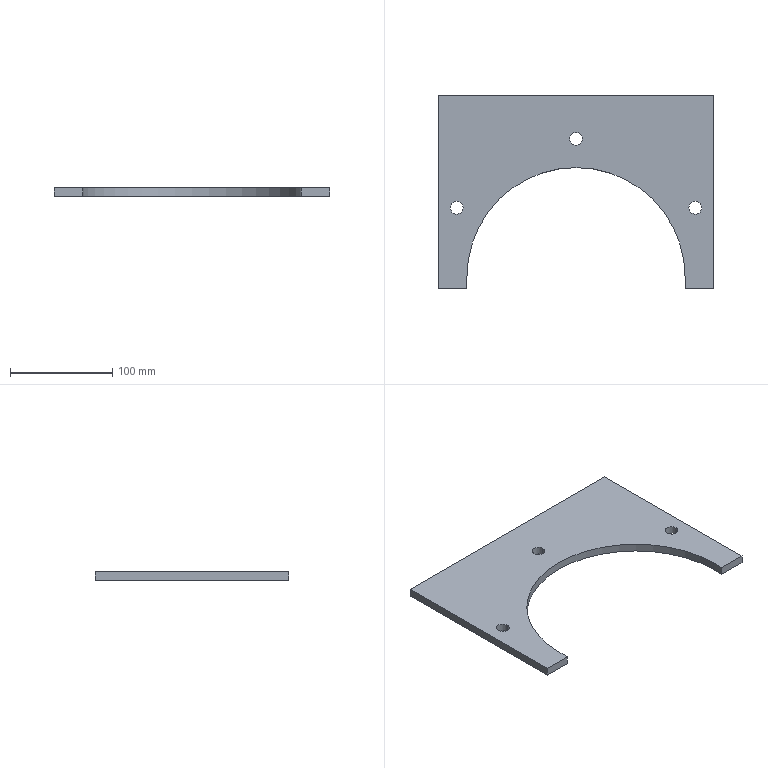Part | SolidWorks | features Cut 1, Extrusion 1 | 1 solid | 16 faces | box 270 x 190 x 8 mm | volume 243470 mm3 | plane 9 | cylinder 7 | commonest cylinder face diameters 12.5 x6 213.7 x1
STEP:
#1=CARTESIAN_POINT('',(123.163,67.5,8.));
#2=VERTEX_POINT('',#1);
#3=CARTESIAN_POINT('',(110.663,67.5,8.));
#4=VERTEX_POINT('',#3);
#5=CARTESIAN_POINT('',(116.913,67.5,8.));
#6=DIRECTION('',(0.,0.,-1.));
#7=DIRECTION('',(-1.,0.,0.));
#8=AXIS2_PLACEMENT_3D('',#5,#6,#7);
#9=CIRCLE('',#8,6.25);
#10=EDGE_CURVE('',#2,#4,#9,.T.);
#11=ORIENTED_EDGE('',*,*,#10,.F.);
#12=CARTESIAN_POINT('',(123.163,67.5,0.));
#13=VERTEX_POINT('',#12);
#14=CARTESIAN_POINT('',(123.163,67.5,8.));
#15=DIRECTION('',(0.,0.,-1.));
#16=VECTOR('',#15,1000.);
#17=LINE('',#14,#16);
#18=EDGE_CURVE('',#2,#13,#17,.T.);
#19=ORIENTED_EDGE('',*,*,#18,.T.);
#20=CARTESIAN_POINT('',(110.663,67.5,0.));
#21=VERTEX_POINT('',#20);
#22=CARTESIAN_POINT('',(116.913,67.5,0.));
#23=DIRECTION('',(0.,0.,-1.));
#24=DIRECTION('',(-1.,0.,0.));
#25=AXIS2_PLACEMENT_3D('',#22,#23,#24);
#26=CIRCLE('',#25,6.25);
#27=EDGE_CURVE('',#13,#21,#26,.T.);
#28=ORIENTED_EDGE('',*,*,#27,.T.);
#29=CARTESIAN_POINT('',(110.663,67.5,8.));
#30=DIRECTION('',(0.,0.,-1.));
#31=VECTOR('',#30,1000.);
#32=LINE('',#29,#31);
#33=EDGE_CURVE('',#4,#21,#32,.T.);
#34=ORIENTED_EDGE('',*,*,#33,.F.);
#35=EDGE_LOOP('',(#11,#19,#28,#34));
#36=FACE_OUTER_BOUND('',#35,.T.);
#37=CARTESIAN_POINT('',(116.913,67.5,8.));
#38=DIRECTION('',(0.,0.,-1.));
#39=DIRECTION('',(-1.,0.,0.));
#40=AXIS2_PLACEMENT_3D('',#37,#38,#39);
#41=CYLINDRICAL_SURFACE('',#40,6.25);
#42=ADVANCED_FACE('',(#36),#41,.F.);
#43=CARTESIAN_POINT('',(-110.663,67.5,8.));
#44=VERTEX_POINT('',#43);
#45=CARTESIAN_POINT('',(-123.163,67.5,8.));
#46=VERTEX_POINT('',#45);
#47=CARTESIAN_POINT('',(-116.913,67.5,8.));
#48=DIRECTION('',(0.,0.,-1.));
#49=DIRECTION('',(-1.,0.,0.));
#50=AXIS2_PLACEMENT_3D('',#47,#48,#49);
#51=CIRCLE('',#50,6.25);
#52=EDGE_CURVE('',#44,#46,#51,.T.);
#53=ORIENTED_EDGE('',*,*,#52,.F.);
#54=CARTESIAN_POINT('',(-110.663,67.5,0.));
#55=VERTEX_POINT('',#54);
#56=CARTESIAN_POINT('',(-110.663,67.5,8.));
#57=DIRECTION('',(0.,0.,-1.));
#58=VECTOR('',#57,1000.);
#59=LINE('',#56,#58);
#60=EDGE_CURVE('',#44,#55,#59,.T.);
#61=ORIENTED_EDGE('',*,*,#60,.T.);
#62=CARTESIAN_POINT('',(-123.163,67.5,0.));
#63=VERTEX_POINT('',#62);
#64=CARTESIAN_POINT('',(-116.913,67.5,0.));
#65=DIRECTION('',(0.,0.,-1.));
#66=DIRECTION('',(-1.,0.,0.));
#67=AXIS2_PLACEMENT_3D('',#64,#65,#66);
#68=CIRCLE('',#67,6.25);
#69=EDGE_CURVE('',#55,#63,#68,.T.);
#70=ORIENTED_EDGE('',*,*,#69,.T.);
#71=CARTESIAN_POINT('',(-123.163,67.5,8.));
#72=DIRECTION('',(0.,0.,-1.));
#73=VECTOR('',#72,1000.);
#74=LINE('',#71,#73);
#75=EDGE_CURVE('',#46,#63,#74,.T.);
#76=ORIENTED_EDGE('',*,*,#75,.F.);
#77=EDGE_LOOP('',(#53,#61,#70,#76));
#78=FACE_OUTER_BOUND('',#77,.T.);
#79=CARTESIAN_POINT('',(-116.913,67.5,8.));
#80=DIRECTION('',(0.,0.,-1.));
#81=DIRECTION('',(-1.,0.,0.));
#82=AXIS2_PLACEMENT_3D('',#79,#80,#81);
#83=CYLINDRICAL_SURFACE('',#82,6.25);
#84=ADVANCED_FACE('',(#78),#83,.F.);
#85=CARTESIAN_POINT('',(6.25,135.,8.));
#86=VERTEX_POINT('',#85);
#87=CARTESIAN_POINT('',(-6.25,135.,8.));
#88=VERTEX_POINT('',#87);
#89=CARTESIAN_POINT('',(0.,135.,8.));
#90=DIRECTION('',(0.,0.,-1.));
#91=DIRECTION('',(-1.,0.,0.));
#92=AXIS2_PLACEMENT_3D('',#89,#90,#91);
#93=CIRCLE('',#92,6.25);
#94=EDGE_CURVE('',#86,#88,#93,.T.);
#95=ORIENTED_EDGE('',*,*,#94,.F.);
#96=CARTESIAN_POINT('',(6.25,135.,0.));
#97=VERTEX_POINT('',#96);
#98=CARTESIAN_POINT('',(6.25,135.,8.));
#99=DIRECTION('',(0.,0.,-1.));
#100=VECTOR('',#99,1000.);
#101=LINE('',#98,#100);
#102=EDGE_CURVE('',#86,#97,#101,.T.);
#103=ORIENTED_EDGE('',*,*,#102,.T.);
#104=CARTESIAN_POINT('',(-6.25,135.,0.));
#105=VERTEX_POINT('',#104);
#106=CARTESIAN_POINT('',(0.,135.,0.));
#107=DIRECTION('',(0.,0.,-1.));
#108=DIRECTION('',(-1.,0.,0.));
#109=AXIS2_PLACEMENT_3D('',#106,#107,#108);
#110=CIRCLE('',#109,6.25);
#111=EDGE_CURVE('',#97,#105,#110,.T.);
#112=ORIENTED_EDGE('',*,*,#111,.T.);
#113=CARTESIAN_POINT('',(-6.25,135.,8.));
#114=DIRECTION('',(0.,0.,-1.));
#115=VECTOR('',#114,1000.);
#116=LINE('',#113,#115);
#117=EDGE_CURVE('',#88,#105,#116,.T.);
#118=ORIENTED_EDGE('',*,*,#117,.F.);
#119=EDGE_LOOP('',(#95,#103,#112,#118));
#120=FACE_OUTER_BOUND('',#119,.T.);
#121=CARTESIAN_POINT('',(0.,135.,8.));
#122=DIRECTION('',(0.,0.,-1.));
#123=DIRECTION('',(-1.,0.,0.));
#124=AXIS2_PLACEMENT_3D('',#121,#122,#123);
#125=CYLINDRICAL_SURFACE('',#124,6.25);
#126=ADVANCED_FACE('',(#120),#125,.F.);
#127=CARTESIAN_POINT('',(-106.85,0.,0.));
#128=VERTEX_POINT('',#127);
#129=CARTESIAN_POINT('',(106.85,0.,0.));
#130=VERTEX_POINT('',#129);
#131=CARTESIAN_POINT('',(0.,0.,0.));
#132=DIRECTION('',(0.,0.,-1.));
#133=DIRECTION('',(1.,0.,0.));
#134=AXIS2_PLACEMENT_3D('',#131,#132,#133);
#135=CIRCLE('',#134,106.85);
#136=EDGE_CURVE('',#128,#130,#135,.T.);
#137=ORIENTED_EDGE('',*,*,#136,.T.);
#138=CARTESIAN_POINT('',(106.85,0.,8.));
#139=VERTEX_POINT('',#138);
#140=CARTESIAN_POINT('',(106.85,0.,8.));
#141=DIRECTION('',(0.,0.,-1.));
#142=VECTOR('',#141,1000.);
#143=LINE('',#140,#142);
#144=EDGE_CURVE('',#139,#130,#143,.T.);
#145=ORIENTED_EDGE('',*,*,#144,.F.);
#146=CARTESIAN_POINT('',(-106.85,0.,8.));
#147=VERTEX_POINT('',#146);
#148=CARTESIAN_POINT('',(0.,0.,8.));
#149=DIRECTION('',(0.,0.,-1.));
#150=DIRECTION('',(1.,0.,0.));
#151=AXIS2_PLACEMENT_3D('',#148,#149,#150);
#152=CIRCLE('',#151,106.85);
#153=EDGE_CURVE('',#147,#139,#152,.T.);
#154=ORIENTED_EDGE('',*,*,#153,.F.);
#155=CARTESIAN_POINT('',(-106.85,0.,8.));
#156=DIRECTION('',(0.,0.,-1.));
#157=VECTOR('',#156,1000.);
#158=LINE('',#155,#157);
#159=EDGE_CURVE('',#147,#128,#158,.T.);
#160=ORIENTED_EDGE('',*,*,#159,.T.);
#161=EDGE_LOOP('',(#137,#145,#154,#160));
#162=FACE_OUTER_BOUND('',#161,.T.);
#163=CARTESIAN_POINT('',(0.,0.,8.));
#164=DIRECTION('',(0.,0.,-1.));
#165=DIRECTION('',(-1.,0.,0.));
#166=AXIS2_PLACEMENT_3D('',#163,#164,#165);
#167=CYLINDRICAL_SURFACE('',#166,106.85);
#168=ADVANCED_FACE('',(#162),#167,.F.);
#169=CARTESIAN_POINT('',(106.85,-12.,0.));
#170=VERTEX_POINT('',#169);
#171=CARTESIAN_POINT('',(106.85,0.,0.));
#172=DIRECTION('',(0.,-1.,0.));
#173=VECTOR('',#172,1000.);
#174=LINE('',#171,#173);
#175=EDGE_CURVE('',#130,#170,#174,.T.);
#176=ORIENTED_EDGE('',*,*,#175,.T.);
#177=CARTESIAN_POINT('',(106.85,-12.,8.));
#178=VERTEX_POINT('',#177);
#179=CARTESIAN_POINT('',(106.85,-12.,8.));
#180=DIRECTION('',(0.,0.,-1.));
#181=VECTOR('',#180,1000.);
#182=LINE('',#179,#181);
#183=EDGE_CURVE('',#178,#170,#182,.T.);
#184=ORIENTED_EDGE('',*,*,#183,.F.);
#185=CARTESIAN_POINT('',(106.85,0.,8.));
#186=DIRECTION('',(0.,-1.,0.));
#187=VECTOR('',#186,1000.);
#188=LINE('',#185,#187);
#189=EDGE_CURVE('',#139,#178,#188,.T.);
#190=ORIENTED_EDGE('',*,*,#189,.F.);
#191=ORIENTED_EDGE('',*,*,#144,.T.);
#192=EDGE_LOOP('',(#176,#184,#190,#191));
#193=FACE_OUTER_BOUND('',#192,.T.);
#194=CARTESIAN_POINT('',(106.85,0.,8.));
#195=DIRECTION('',(1.,0.,0.));
#196=DIRECTION('',(0.,0.,-1.));
#197=AXIS2_PLACEMENT_3D('',#194,#195,#196);
#198=PLANE('',#197);
#199=ADVANCED_FACE('',(#193),#198,.F.);
#200=CARTESIAN_POINT('',(135.,-12.,0.));
#201=VERTEX_POINT('',#200);
#202=CARTESIAN_POINT('',(106.85,-12.,0.));
#203=DIRECTION('',(1.,0.,0.));
#204=VECTOR('',#203,1000.);
#205=LINE('',#202,#204);
#206=EDGE_CURVE('',#170,#201,#205,.T.);
#207=ORIENTED_EDGE('',*,*,#206,.T.);
#208=CARTESIAN_POINT('',(135.,-12.,8.));
#209=VERTEX_POINT('',#208);
#210=CARTESIAN_POINT('',(135.,-12.,8.));
#211=DIRECTION('',(0.,0.,-1.));
#212=VECTOR('',#211,1000.);
#213=LINE('',#210,#212);
#214=EDGE_CURVE('',#209,#201,#213,.T.);
#215=ORIENTED_EDGE('',*,*,#214,.F.);
#216=CARTESIAN_POINT('',(106.85,-12.,8.));
#217=DIRECTION('',(1.,0.,0.));
#218=VECTOR('',#217,1000.);
#219=LINE('',#216,#218);
#220=EDGE_CURVE('',#178,#209,#219,.T.);
#221=ORIENTED_EDGE('',*,*,#220,.F.);
#222=ORIENTED_EDGE('',*,*,#183,.T.);
#223=EDGE_LOOP('',(#207,#215,#221,#222));
#224=FACE_OUTER_BOUND('',#223,.T.);
#225=CARTESIAN_POINT('',(106.85,-12.,8.));
#226=DIRECTION('',(0.,1.,0.));
#227=DIRECTION('',(-1.,0.,0.));
#228=AXIS2_PLACEMENT_3D('',#225,#226,#227);
#229=PLANE('',#228);
#230=ADVANCED_FACE('',(#224),#229,.F.);
#231=CARTESIAN_POINT('',(135.,178.,0.));
#232=VERTEX_POINT('',#231);
#233=CARTESIAN_POINT('',(135.,-12.,0.));
#234=DIRECTION('',(0.,1.,0.));
#235=VECTOR('',#234,1000.);
#236=LINE('',#233,#235);
#237=EDGE_CURVE('',#201,#232,#236,.T.);
#238=ORIENTED_EDGE('',*,*,#237,.T.);
#239=CARTESIAN_POINT('',(135.,178.,8.));
#240=VERTEX_POINT('',#239);
#241=CARTESIAN_POINT('',(135.,178.,8.));
#242=DIRECTION('',(0.,0.,-1.));
#243=VECTOR('',#242,1000.);
#244=LINE('',#241,#243);
#245=EDGE_CURVE('',#240,#232,#244,.T.);
#246=ORIENTED_EDGE('',*,*,#245,.F.);
#247=CARTESIAN_POINT('',(135.,-12.,8.));
#248=DIRECTION('',(0.,1.,0.));
#249=VECTOR('',#248,1000.);
#250=LINE('',#247,#249);
#251=EDGE_CURVE('',#209,#240,#250,.T.);
#252=ORIENTED_EDGE('',*,*,#251,.F.);
#253=ORIENTED_EDGE('',*,*,#214,.T.);
#254=EDGE_LOOP('',(#238,#246,#252,#253));
#255=FACE_OUTER_BOUND('',#254,.T.);
#256=CARTESIAN_POINT('',(135.,-12.,8.));
#257=DIRECTION('',(-1.,0.,0.));
#258=DIRECTION('',(0.,-1.,0.));
#259=AXIS2_PLACEMENT_3D('',#256,#257,#258);
#260=PLANE('',#259);
#261=ADVANCED_FACE('',(#255),#260,.F.);
#262=CARTESIAN_POINT('',(-135.,178.,0.));
#263=VERTEX_POINT('',#262);
#264=CARTESIAN_POINT('',(135.,178.,0.));
#265=DIRECTION('',(-1.,0.,0.));
#266=VECTOR('',#265,1000.);
#267=LINE('',#264,#266);
#268=EDGE_CURVE('',#232,#263,#267,.T.);
#269=ORIENTED_EDGE('',*,*,#268,.T.);
#270=CARTESIAN_POINT('',(-135.,178.,8.));
#271=VERTEX_POINT('',#270);
#272=CARTESIAN_POINT('',(-135.,178.,8.));
#273=DIRECTION('',(0.,0.,-1.));
#274=VECTOR('',#273,1000.);
#275=LINE('',#272,#274);
#276=EDGE_CURVE('',#271,#263,#275,.T.);
#277=ORIENTED_EDGE('',*,*,#276,.F.);
#278=CARTESIAN_POINT('',(135.,178.,8.));
#279=DIRECTION('',(-1.,0.,0.));
#280=VECTOR('',#279,1000.);
#281=LINE('',#278,#280);
#282=EDGE_CURVE('',#240,#271,#281,.T.);
#283=ORIENTED_EDGE('',*,*,#282,.F.);
#284=ORIENTED_EDGE('',*,*,#245,.T.);
#285=EDGE_LOOP('',(#269,#277,#283,#284));
#286=FACE_OUTER_BOUND('',#285,.T.);
#287=CARTESIAN_POINT('',(135.,178.,8.));
#288=DIRECTION('',(0.,-1.,0.));
#289=DIRECTION('',(0.,0.,-1.));
#290=AXIS2_PLACEMENT_3D('',#287,#288,#289);
#291=PLANE('',#290);
#292=ADVANCED_FACE('',(#286),#291,.F.);
#293=CARTESIAN_POINT('',(-135.,-12.,0.));
#294=VERTEX_POINT('',#293);
#295=CARTESIAN_POINT('',(-135.,-12.,0.));
#296=DIRECTION('',(0.,-1.,0.));
#297=VECTOR('',#296,1000.);
#298=LINE('',#295,#297);
#299=EDGE_CURVE('',#263,#294,#298,.T.);
#300=ORIENTED_EDGE('',*,*,#299,.T.);
#301=CARTESIAN_POINT('',(-135.,-12.,8.));
#302=VERTEX_POINT('',#301);
#303=CARTESIAN_POINT('',(-135.,-12.,8.));
#304=DIRECTION('',(0.,0.,-1.));
#305=VECTOR('',#304,1000.);
#306=LINE('',#303,#305);
#307=EDGE_CURVE('',#302,#294,#306,.T.);
#308=ORIENTED_EDGE('',*,*,#307,.F.);
#309=CARTESIAN_POINT('',(-135.,-12.,8.));
#310=DIRECTION('',(0.,-1.,0.));
#311=VECTOR('',#310,1000.);
#312=LINE('',#309,#311);
#313=EDGE_CURVE('',#271,#302,#312,.T.);
#314=ORIENTED_EDGE('',*,*,#313,.F.);
#315=ORIENTED_EDGE('',*,*,#276,.T.);
#316=EDGE_LOOP('',(#300,#308,#314,#315));
#317=FACE_OUTER_BOUND('',#316,.T.);
#318=CARTESIAN_POINT('',(-135.,-12.,8.));
#319=DIRECTION('',(1.,0.,0.));
#320=DIRECTION('',(0.,0.,-1.));
#321=AXIS2_PLACEMENT_3D('',#318,#319,#320);
#322=PLANE('',#321);
#323=ADVANCED_FACE('',(#317),#322,.F.);
#324=CARTESIAN_POINT('',(-106.85,-12.,0.));
#325=VERTEX_POINT('',#324);
#326=CARTESIAN_POINT('',(-106.85,-12.,0.));
#327=DIRECTION('',(1.,0.,0.));
#328=VECTOR('',#327,1000.);
#329=LINE('',#326,#328);
#330=EDGE_CURVE('',#294,#325,#329,.T.);
#331=ORIENTED_EDGE('',*,*,#330,.T.);
#332=CARTESIAN_POINT('',(-106.85,-12.,8.));
#333=VERTEX_POINT('',#332);
#334=CARTESIAN_POINT('',(-106.85,-12.,8.));
#335=DIRECTION('',(0.,0.,-1.));
#336=VECTOR('',#335,1000.);
#337=LINE('',#334,#336);
#338=EDGE_CURVE('',#333,#325,#337,.T.);
#339=ORIENTED_EDGE('',*,*,#338,.F.);
#340=CARTESIAN_POINT('',(-106.85,-12.,8.));
#341=DIRECTION('',(1.,0.,0.));
#342=VECTOR('',#341,1000.);
#343=LINE('',#340,#342);
#344=EDGE_CURVE('',#302,#333,#343,.T.);
#345=ORIENTED_EDGE('',*,*,#344,.F.);
#346=ORIENTED_EDGE('',*,*,#307,.T.);
#347=EDGE_LOOP('',(#331,#339,#345,#346));
#348=FACE_OUTER_BOUND('',#347,.T.);
#349=CARTESIAN_POINT('',(-106.85,-12.,8.));
#350=DIRECTION('',(0.,1.,0.));
#351=DIRECTION('',(-1.,0.,0.));
#352=AXIS2_PLACEMENT_3D('',#349,#350,#351);
#353=PLANE('',#352);
#354=ADVANCED_FACE('',(#348),#353,.F.);
#355=CARTESIAN_POINT('',(-106.85,0.,0.));
#356=DIRECTION('',(0.,1.,0.));
#357=VECTOR('',#356,1000.);
#358=LINE('',#355,#357);
#359=EDGE_CURVE('',#325,#128,#358,.T.);
#360=ORIENTED_EDGE('',*,*,#359,.T.);
#361=ORIENTED_EDGE('',*,*,#159,.F.);
#362=CARTESIAN_POINT('',(-106.85,0.,8.));
#363=DIRECTION('',(0.,1.,0.));
#364=VECTOR('',#363,1000.);
#365=LINE('',#362,#364);
#366=EDGE_CURVE('',#333,#147,#365,.T.);
#367=ORIENTED_EDGE('',*,*,#366,.F.);
#368=ORIENTED_EDGE('',*,*,#338,.T.);
#369=EDGE_LOOP('',(#360,#361,#367,#368));
#370=FACE_OUTER_BOUND('',#369,.T.);
#371=CARTESIAN_POINT('',(-106.85,0.,8.));
#372=DIRECTION('',(-1.,0.,0.));
#373=DIRECTION('',(0.,0.,1.));
#374=AXIS2_PLACEMENT_3D('',#371,#372,#373);
#375=PLANE('',#374);
#376=ADVANCED_FACE('',(#370),#375,.F.);
#377=CARTESIAN_POINT('',(116.913,67.5,8.));
#378=DIRECTION('',(0.,0.,-1.));
#379=DIRECTION('',(-1.,0.,0.));
#380=AXIS2_PLACEMENT_3D('',#377,#378,#379);
#381=CIRCLE('',#380,6.25);
#382=EDGE_CURVE('',#4,#2,#381,.T.);
#383=ORIENTED_EDGE('',*,*,#382,.T.);
#384=ORIENTED_EDGE('',*,*,#10,.T.);
#385=EDGE_LOOP('',(#383,#384));
#386=FACE_BOUND('',#385,.T.);
#387=CARTESIAN_POINT('',(-116.913,67.5,8.));
#388=DIRECTION('',(0.,0.,-1.));
#389=DIRECTION('',(-1.,0.,0.));
#390=AXIS2_PLACEMENT_3D('',#387,#388,#389);
#391=CIRCLE('',#390,6.25);
#392=EDGE_CURVE('',#46,#44,#391,.T.);
#393=ORIENTED_EDGE('',*,*,#392,.T.);
#394=ORIENTED_EDGE('',*,*,#52,.T.);
#395=EDGE_LOOP('',(#393,#394));
#396=FACE_BOUND('',#395,.T.);
#397=CARTESIAN_POINT('',(0.,135.,8.));
#398=DIRECTION('',(0.,0.,-1.));
#399=DIRECTION('',(-1.,0.,0.));
#400=AXIS2_PLACEMENT_3D('',#397,#398,#399);
#401=CIRCLE('',#400,6.25);
#402=EDGE_CURVE('',#88,#86,#401,.T.);
#403=ORIENTED_EDGE('',*,*,#402,.T.);
#404=ORIENTED_EDGE('',*,*,#94,.T.);
#405=EDGE_LOOP('',(#403,#404));
#406=FACE_BOUND('',#405,.T.);
#407=ORIENTED_EDGE('',*,*,#153,.T.);
#408=ORIENTED_EDGE('',*,*,#189,.T.);
#409=ORIENTED_EDGE('',*,*,#220,.T.);
#410=ORIENTED_EDGE('',*,*,#251,.T.);
#411=ORIENTED_EDGE('',*,*,#282,.T.);
#412=ORIENTED_EDGE('',*,*,#313,.T.);
#413=ORIENTED_EDGE('',*,*,#344,.T.);
#414=ORIENTED_EDGE('',*,*,#366,.T.);
#415=EDGE_LOOP('',(#407,#408,#409,#410,#411,#412,#413,#414));
#416=FACE_OUTER_BOUND('',#415,.T.);
#417=CARTESIAN_POINT('',(0.,0.,8.));
#418=DIRECTION('',(0.,0.,1.));
#419=DIRECTION('',(1.,0.,0.));
#420=AXIS2_PLACEMENT_3D('',#417,#418,#419);
#421=PLANE('',#420);
#422=ADVANCED_FACE('',(#386,#396,#406,#416),#421,.T.);
#423=CARTESIAN_POINT('',(116.913,67.5,0.));
#424=DIRECTION('',(0.,0.,-1.));
#425=DIRECTION('',(-1.,0.,0.));
#426=AXIS2_PLACEMENT_3D('',#423,#424,#425);
#427=CIRCLE('',#426,6.25);
#428=EDGE_CURVE('',#21,#13,#427,.T.);
#429=ORIENTED_EDGE('',*,*,#428,.F.);
#430=ORIENTED_EDGE('',*,*,#27,.F.);
#431=EDGE_LOOP('',(#429,#430));
#432=FACE_BOUND('',#431,.T.);
#433=CARTESIAN_POINT('',(-116.913,67.5,0.));
#434=DIRECTION('',(0.,0.,-1.));
#435=DIRECTION('',(-1.,0.,0.));
#436=AXIS2_PLACEMENT_3D('',#433,#434,#435);
#437=CIRCLE('',#436,6.25);
#438=EDGE_CURVE('',#63,#55,#437,.T.);
#439=ORIENTED_EDGE('',*,*,#438,.F.);
#440=ORIENTED_EDGE('',*,*,#69,.F.);
#441=EDGE_LOOP('',(#439,#440));
#442=FACE_BOUND('',#441,.T.);
#443=CARTESIAN_POINT('',(0.,135.,0.));
#444=DIRECTION('',(0.,0.,-1.));
#445=DIRECTION('',(-1.,0.,0.));
#446=AXIS2_PLACEMENT_3D('',#443,#444,#445);
#447=CIRCLE('',#446,6.25);
#448=EDGE_CURVE('',#105,#97,#447,.T.);
#449=ORIENTED_EDGE('',*,*,#448,.F.);
#450=ORIENTED_EDGE('',*,*,#111,.F.);
#451=EDGE_LOOP('',(#449,#450));
#452=FACE_BOUND('',#451,.T.);
#453=ORIENTED_EDGE('',*,*,#136,.F.);
#454=ORIENTED_EDGE('',*,*,#359,.F.);
#455=ORIENTED_EDGE('',*,*,#330,.F.);
#456=ORIENTED_EDGE('',*,*,#299,.F.);
#457=ORIENTED_EDGE('',*,*,#268,.F.);
#458=ORIENTED_EDGE('',*,*,#237,.F.);
#459=ORIENTED_EDGE('',*,*,#206,.F.);
#460=ORIENTED_EDGE('',*,*,#175,.F.);
#461=EDGE_LOOP('',(#453,#454,#455,#456,#457,#458,#459,#460));
#462=FACE_OUTER_BOUND('',#461,.T.);
#463=CARTESIAN_POINT('',(0.,0.,0.));
#464=DIRECTION('',(0.,0.,1.));
#465=DIRECTION('',(1.,0.,0.));
#466=AXIS2_PLACEMENT_3D('',#463,#464,#465);
#467=PLANE('',#466);
#468=ADVANCED_FACE('',(#432,#442,#452,#462),#467,.F.);
#469=ORIENTED_EDGE('',*,*,#102,.F.);
#470=ORIENTED_EDGE('',*,*,#402,.F.);
#471=ORIENTED_EDGE('',*,*,#117,.T.);
#472=ORIENTED_EDGE('',*,*,#448,.T.);
#473=EDGE_LOOP('',(#469,#470,#471,#472));
#474=FACE_OUTER_BOUND('',#473,.T.);
#475=CARTESIAN_POINT('',(0.,135.,8.));
#476=DIRECTION('',(0.,0.,-1.));
#477=DIRECTION('',(-1.,0.,0.));
#478=AXIS2_PLACEMENT_3D('',#475,#476,#477);
#479=CYLINDRICAL_SURFACE('',#478,6.25);
#480=ADVANCED_FACE('',(#474),#479,.F.);
#481=ORIENTED_EDGE('',*,*,#60,.F.);
#482=ORIENTED_EDGE('',*,*,#392,.F.);
#483=ORIENTED_EDGE('',*,*,#75,.T.);
#484=ORIENTED_EDGE('',*,*,#438,.T.);
#485=EDGE_LOOP('',(#481,#482,#483,#484));
#486=FACE_OUTER_BOUND('',#485,.T.);
#487=CARTESIAN_POINT('',(-116.913,67.5,8.));
#488=DIRECTION('',(0.,0.,-1.));
#489=DIRECTION('',(-1.,0.,0.));
#490=AXIS2_PLACEMENT_3D('',#487,#488,#489);
#491=CYLINDRICAL_SURFACE('',#490,6.25);
#492=ADVANCED_FACE('',(#486),#491,.F.);
#493=ORIENTED_EDGE('',*,*,#18,.F.);
#494=ORIENTED_EDGE('',*,*,#382,.F.);
#495=ORIENTED_EDGE('',*,*,#33,.T.);
#496=ORIENTED_EDGE('',*,*,#428,.T.);
#497=EDGE_LOOP('',(#493,#494,#495,#496));
#498=FACE_OUTER_BOUND('',#497,.T.);
#499=CARTESIAN_POINT('',(116.913,67.5,8.));
#500=DIRECTION('',(0.,0.,-1.));
#501=DIRECTION('',(-1.,0.,0.));
#502=AXIS2_PLACEMENT_3D('',#499,#500,#501);
#503=CYLINDRICAL_SURFACE('',#502,6.25);
#504=ADVANCED_FACE('',(#498),#503,.F.);
#505=CLOSED_SHELL('',(#42,#84,#126,#168,#199,#230,#261,#292,#323,#354,#376,#422,#468,#480,#492,#504));
#506=MANIFOLD_SOLID_BREP('',#505);
#507=CARTESIAN_POINT('',(0.,0.,0.));
#508=DIRECTION('',(0.,0.,1.));
#509=DIRECTION('',(1.,0.,0.));
#510=AXIS2_PLACEMENT_3D('',#507,#508,#509);
#511=(LENGTH_UNIT()NAMED_UNIT(*)SI_UNIT(.MILLI.,.METRE.));
#512=UNCERTAINTY_MEASURE_WITH_UNIT(LENGTH_MEASURE(0.00001),#511,'','');
#513=(NAMED_UNIT(*)PLANE_ANGLE_UNIT()SI_UNIT($,.RADIAN.));
#514=(NAMED_UNIT(*)SI_UNIT($,.STERADIAN.)SOLID_ANGLE_UNIT());
#515=(GEOMETRIC_REPRESENTATION_CONTEXT(3)GLOBAL_UNCERTAINTY_ASSIGNED_CONTEXT((#512))GLOBAL_UNIT_ASSIGNED_CONTEXT((#511,#513,#514))REPRESENTATION_CONTEXT('',''));
#516=ADVANCED_BREP_SHAPE_REPRESENTATION('',(#506,#510),#515);